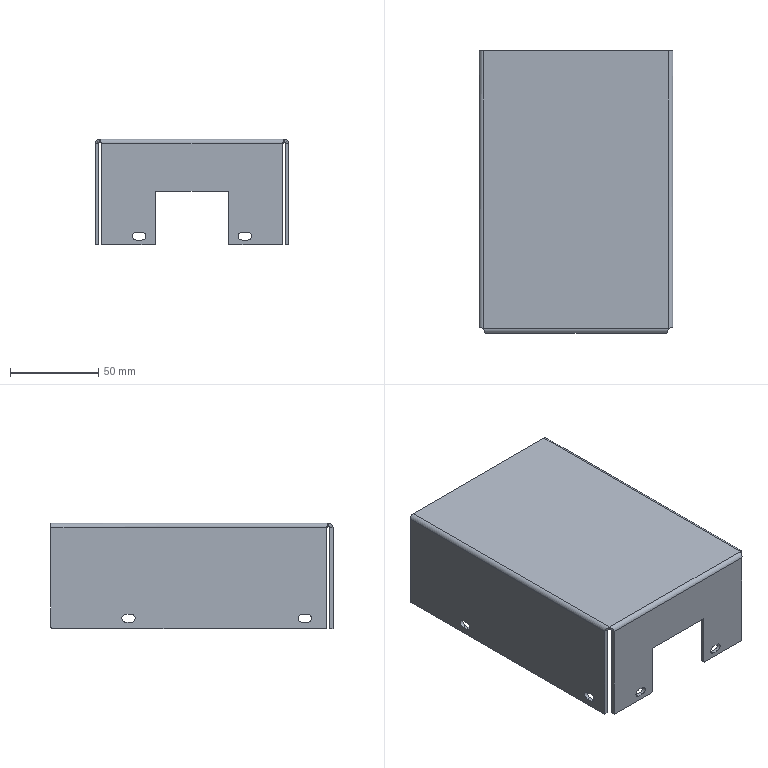Part | STEP file | 1 solid | 62 faces | box 110 x 160 x 60 mm | volume 79904 mm3 | plane 36 | cylinder 22 | spline 4 | commonest cylinder face diameters 4.5 x12 2 x4 1 x3 5 x3